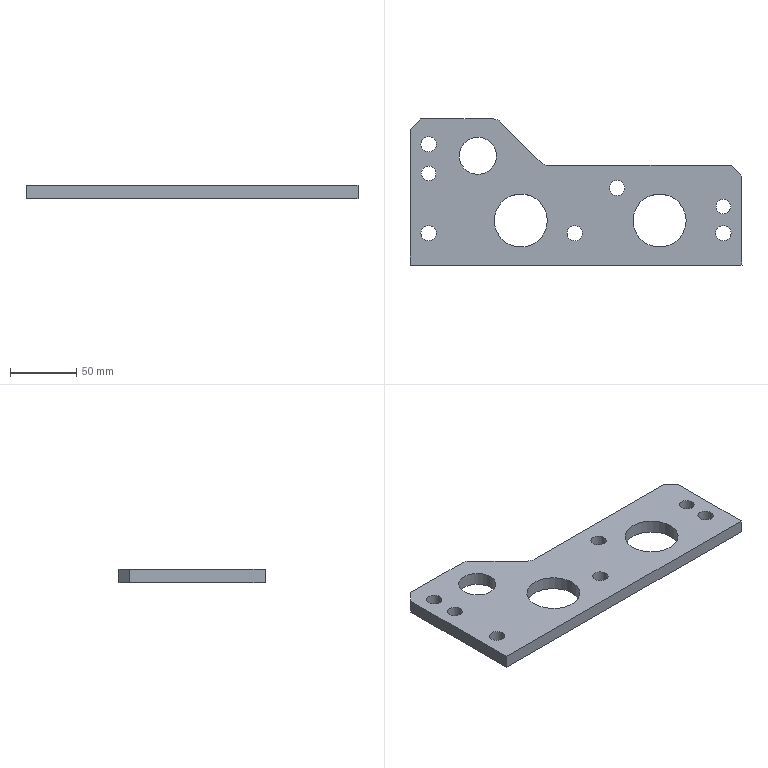Part | STEP file | lll_id4274_x_t | 1 solid | 22 faces | box 250 x 110 x 10 mm | volume 177692 mm3 | cylinder 12 | plane 10 | commonest cylinder face diameters 11.509 x5 11 x2 16 x2 40 x2 28 x1
STEP:
#1=CARTESIAN_POINT('',(3220.278,-130.093,-35.));
#2=VERTEX_POINT('',#1);
#3=CARTESIAN_POINT('',(3220.278,-130.093,-45.));
#4=VERTEX_POINT('',#3);
#5=CARTESIAN_POINT('',(3220.278,-130.093,-35.));
#6=DIRECTION('',(0.,0.,-1.));
#7=VECTOR('',#6,1.);
#8=LINE('',#5,#7);
#9=EDGE_CURVE('',#2,#4,#8,.T.);
#10=ORIENTED_EDGE('',*,*,#9,.F.);
#11=CARTESIAN_POINT('',(3250.592,-160.407,-35.));
#12=VERTEX_POINT('',#11);
#13=CARTESIAN_POINT('',(3285.935,-195.75,-35.));
#14=DIRECTION('',(0.7071,-0.7071,0.));
#15=VECTOR('',#14,1.);
#16=LINE('',#13,#15);
#17=EDGE_CURVE('',#2,#12,#16,.T.);
#18=ORIENTED_EDGE('',*,*,#17,.T.);
#19=CARTESIAN_POINT('',(3250.592,-160.407,-45.));
#20=VERTEX_POINT('',#19);
#21=CARTESIAN_POINT('',(3250.592,-160.407,-35.));
#22=DIRECTION('',(0.,0.,-1.));
#23=VECTOR('',#22,1.);
#24=LINE('',#21,#23);
#25=EDGE_CURVE('',#12,#20,#24,.T.);
#26=ORIENTED_EDGE('',*,*,#25,.T.);
#27=CARTESIAN_POINT('',(3434.56,-344.374,-45.));
#28=DIRECTION('',(0.7071,-0.7071,0.));
#29=VECTOR('',#28,1.);
#30=LINE('',#27,#29);
#31=EDGE_CURVE('',#4,#20,#30,.T.);
#32=ORIENTED_EDGE('',*,*,#31,.F.);
#33=EDGE_LOOP('',(#10,#18,#26,#32));
#34=FACE_OUTER_BOUND('',#33,.T.);
#35=CARTESIAN_POINT('',(3285.935,-195.75,-35.));
#36=DIRECTION('',(-0.7071,-0.7071,0.));
#37=DIRECTION('',(-0.7071,0.7071,0.));
#38=AXIS2_PLACEMENT_3D('',#35,#36,#37);
#39=PLANE('',#38);
#40=ADVANCED_FACE('',(#34),#39,.F.);
#41=ORIENTED_EDGE('',*,*,#25,.F.);
#42=CARTESIAN_POINT('',(3256.249,-162.75,-35.));
#43=VERTEX_POINT('',#42);
#44=CARTESIAN_POINT('',(3256.249,-154.75,-35.));
#45=DIRECTION('',(0.,0.,1.));
#46=DIRECTION('',(-1.,0.,0.));
#47=AXIS2_PLACEMENT_3D('',#44,#45,#46);
#48=CIRCLE('',#47,8.);
#49=EDGE_CURVE('',#12,#43,#48,.T.);
#50=ORIENTED_EDGE('',*,*,#49,.T.);
#51=CARTESIAN_POINT('',(3256.249,-162.75,-45.));
#52=VERTEX_POINT('',#51);
#53=CARTESIAN_POINT('',(3256.249,-162.75,-35.));
#54=DIRECTION('',(0.,0.,-1.));
#55=VECTOR('',#54,1.);
#56=LINE('',#53,#55);
#57=EDGE_CURVE('',#43,#52,#56,.T.);
#58=ORIENTED_EDGE('',*,*,#57,.T.);
#59=CARTESIAN_POINT('',(3256.249,-154.75,-45.));
#60=DIRECTION('',(0.,0.,1.));
#61=DIRECTION('',(-1.,0.,0.));
#62=AXIS2_PLACEMENT_3D('',#59,#60,#61);
#63=CIRCLE('',#62,8.);
#64=EDGE_CURVE('',#20,#52,#63,.T.);
#65=ORIENTED_EDGE('',*,*,#64,.F.);
#66=EDGE_LOOP('',(#41,#50,#58,#65));
#67=FACE_OUTER_BOUND('',#66,.T.);
#68=CARTESIAN_POINT('',(3256.249,-154.75,-35.));
#69=DIRECTION('',(0.,0.,-1.));
#70=DIRECTION('',(-1.,0.,0.));
#71=AXIS2_PLACEMENT_3D('',#68,#69,#70);
#72=CYLINDRICAL_SURFACE('',#71,8.);
#73=ADVANCED_FACE('',(#67),#72,.F.);
#74=ORIENTED_EDGE('',*,*,#57,.F.);
#75=CARTESIAN_POINT('',(3393.935,-162.75,-35.));
#76=VERTEX_POINT('',#75);
#77=CARTESIAN_POINT('',(3266.435,-162.75,-35.));
#78=DIRECTION('',(-1.,0.,0.));
#79=VECTOR('',#78,1.);
#80=LINE('',#77,#79);
#81=EDGE_CURVE('',#76,#43,#80,.T.);
#82=ORIENTED_EDGE('',*,*,#81,.F.);
#83=CARTESIAN_POINT('',(3393.935,-162.75,-45.));
#84=VERTEX_POINT('',#83);
#85=CARTESIAN_POINT('',(3393.935,-162.75,-35.));
#86=DIRECTION('',(0.,0.,-1.));
#87=VECTOR('',#86,1.);
#88=LINE('',#85,#87);
#89=EDGE_CURVE('',#76,#84,#88,.T.);
#90=ORIENTED_EDGE('',*,*,#89,.T.);
#91=CARTESIAN_POINT('',(3266.435,-162.75,-45.));
#92=DIRECTION('',(-1.,0.,0.));
#93=VECTOR('',#92,1.);
#94=LINE('',#91,#93);
#95=EDGE_CURVE('',#84,#52,#94,.T.);
#96=ORIENTED_EDGE('',*,*,#95,.T.);
#97=EDGE_LOOP('',(#74,#82,#90,#96));
#98=FACE_OUTER_BOUND('',#97,.T.);
#99=CARTESIAN_POINT('',(3266.435,-162.75,-35.));
#100=DIRECTION('',(0.,-1.,0.));
#101=DIRECTION('',(-1.,0.,0.));
#102=AXIS2_PLACEMENT_3D('',#99,#100,#101);
#103=PLANE('',#102);
#104=ADVANCED_FACE('',(#98),#103,.F.);
#105=ORIENTED_EDGE('',*,*,#89,.F.);
#106=CARTESIAN_POINT('',(3401.935,-170.75,-35.));
#107=VERTEX_POINT('',#106);
#108=CARTESIAN_POINT('',(3356.435,-125.25,-35.));
#109=DIRECTION('',(0.7071,-0.7071,0.));
#110=VECTOR('',#109,1.);
#111=LINE('',#108,#110);
#112=EDGE_CURVE('',#76,#107,#111,.T.);
#113=ORIENTED_EDGE('',*,*,#112,.T.);
#114=CARTESIAN_POINT('',(3401.935,-170.75,-45.));
#115=VERTEX_POINT('',#114);
#116=CARTESIAN_POINT('',(3401.935,-170.75,-35.));
#117=DIRECTION('',(0.,0.,-1.));
#118=VECTOR('',#117,1.);
#119=LINE('',#116,#118);
#120=EDGE_CURVE('',#107,#115,#119,.T.);
#121=ORIENTED_EDGE('',*,*,#120,.T.);
#122=CARTESIAN_POINT('',(3505.06,-273.874,-45.));
#123=DIRECTION('',(0.7071,-0.7071,0.));
#124=VECTOR('',#123,1.);
#125=LINE('',#122,#124);
#126=EDGE_CURVE('',#84,#115,#125,.T.);
#127=ORIENTED_EDGE('',*,*,#126,.F.);
#128=EDGE_LOOP('',(#105,#113,#121,#127));
#129=FACE_OUTER_BOUND('',#128,.T.);
#130=CARTESIAN_POINT('',(3356.435,-125.25,-35.));
#131=DIRECTION('',(0.7071,0.7071,0.));
#132=DIRECTION('',(0.7071,-0.7071,0.));
#133=AXIS2_PLACEMENT_3D('',#130,#131,#132);
#134=PLANE('',#133);
#135=ADVANCED_FACE('',(#129),#134,.T.);
#136=ORIENTED_EDGE('',*,*,#120,.F.);
#137=CARTESIAN_POINT('',(3401.935,-237.75,-35.));
#138=VERTEX_POINT('',#137);
#139=CARTESIAN_POINT('',(3401.935,-215.25,-35.));
#140=DIRECTION('',(0.,-1.,0.));
#141=VECTOR('',#140,1.);
#142=LINE('',#139,#141);
#143=EDGE_CURVE('',#107,#138,#142,.T.);
#144=ORIENTED_EDGE('',*,*,#143,.T.);
#145=CARTESIAN_POINT('',(3401.935,-237.75,-45.));
#146=VERTEX_POINT('',#145);
#147=CARTESIAN_POINT('',(3401.935,-237.75,-35.));
#148=DIRECTION('',(0.,0.,-1.));
#149=VECTOR('',#148,1.);
#150=LINE('',#147,#149);
#151=EDGE_CURVE('',#138,#146,#150,.T.);
#152=ORIENTED_EDGE('',*,*,#151,.T.);
#153=CARTESIAN_POINT('',(3401.935,-198.7,-45.));
#154=DIRECTION('',(0.,-1.,0.));
#155=VECTOR('',#154,1.);
#156=LINE('',#153,#155);
#157=EDGE_CURVE('',#115,#146,#156,.T.);
#158=ORIENTED_EDGE('',*,*,#157,.F.);
#159=EDGE_LOOP('',(#136,#144,#152,#158));
#160=FACE_OUTER_BOUND('',#159,.T.);
#161=CARTESIAN_POINT('',(3401.935,-215.25,-35.));
#162=DIRECTION('',(1.,0.,0.));
#163=DIRECTION('',(0.,-1.,0.));
#164=AXIS2_PLACEMENT_3D('',#161,#162,#163);
#165=PLANE('',#164);
#166=ADVANCED_FACE('',(#160),#165,.T.);
#167=ORIENTED_EDGE('',*,*,#151,.F.);
#168=CARTESIAN_POINT('',(3151.935,-237.75,-35.));
#169=VERTEX_POINT('',#168);
#170=CARTESIAN_POINT('',(3266.435,-237.75,-35.));
#171=DIRECTION('',(-1.,0.,0.));
#172=VECTOR('',#171,1.);
#173=LINE('',#170,#172);
#174=EDGE_CURVE('',#138,#169,#173,.T.);
#175=ORIENTED_EDGE('',*,*,#174,.T.);
#176=CARTESIAN_POINT('',(3151.935,-237.75,-45.));
#177=VERTEX_POINT('',#176);
#178=CARTESIAN_POINT('',(3151.935,-237.75,-35.));
#179=DIRECTION('',(0.,0.,-1.));
#180=VECTOR('',#179,1.);
#181=LINE('',#178,#180);
#182=EDGE_CURVE('',#169,#177,#181,.T.);
#183=ORIENTED_EDGE('',*,*,#182,.T.);
#184=CARTESIAN_POINT('',(3580.234,-237.75,-45.));
#185=DIRECTION('',(-1.,0.,0.));
#186=VECTOR('',#185,1.);
#187=LINE('',#184,#186);
#188=EDGE_CURVE('',#146,#177,#187,.T.);
#189=ORIENTED_EDGE('',*,*,#188,.F.);
#190=EDGE_LOOP('',(#167,#175,#183,#189));
#191=FACE_OUTER_BOUND('',#190,.T.);
#192=CARTESIAN_POINT('',(3266.435,-237.75,-35.));
#193=DIRECTION('',(0.,-1.,0.));
#194=DIRECTION('',(-1.,0.,0.));
#195=AXIS2_PLACEMENT_3D('',#192,#193,#194);
#196=PLANE('',#195);
#197=ADVANCED_FACE('',(#191),#196,.T.);
#198=ORIENTED_EDGE('',*,*,#182,.F.);
#199=CARTESIAN_POINT('',(3151.935,-135.75,-35.));
#200=VERTEX_POINT('',#199);
#201=CARTESIAN_POINT('',(3151.935,-215.25,-35.));
#202=DIRECTION('',(0.,1.,0.));
#203=VECTOR('',#202,1.);
#204=LINE('',#201,#203);
#205=EDGE_CURVE('',#169,#200,#204,.T.);
#206=ORIENTED_EDGE('',*,*,#205,.T.);
#207=CARTESIAN_POINT('',(3151.935,-135.75,-45.));
#208=VERTEX_POINT('',#207);
#209=CARTESIAN_POINT('',(3151.935,-135.75,-35.));
#210=DIRECTION('',(0.,0.,-1.));
#211=VECTOR('',#210,1.);
#212=LINE('',#209,#211);
#213=EDGE_CURVE('',#200,#208,#212,.T.);
#214=ORIENTED_EDGE('',*,*,#213,.T.);
#215=CARTESIAN_POINT('',(3151.935,-198.7,-45.));
#216=DIRECTION('',(0.,1.,0.));
#217=VECTOR('',#216,1.);
#218=LINE('',#215,#217);
#219=EDGE_CURVE('',#177,#208,#218,.T.);
#220=ORIENTED_EDGE('',*,*,#219,.F.);
#221=EDGE_LOOP('',(#198,#206,#214,#220));
#222=FACE_OUTER_BOUND('',#221,.T.);
#223=CARTESIAN_POINT('',(3151.935,-215.25,-35.));
#224=DIRECTION('',(-1.,0.,0.));
#225=DIRECTION('',(0.,1.,0.));
#226=AXIS2_PLACEMENT_3D('',#223,#224,#225);
#227=PLANE('',#226);
#228=ADVANCED_FACE('',(#222),#227,.T.);
#229=ORIENTED_EDGE('',*,*,#213,.F.);
#230=CARTESIAN_POINT('',(3159.935,-127.75,-35.));
#231=VERTEX_POINT('',#230);
#232=CARTESIAN_POINT('',(3169.435,-118.25,-35.));
#233=DIRECTION('',(0.7071,0.7071,0.));
#234=VECTOR('',#233,1.);
#235=LINE('',#232,#234);
#236=EDGE_CURVE('',#200,#231,#235,.T.);
#237=ORIENTED_EDGE('',*,*,#236,.T.);
#238=CARTESIAN_POINT('',(3159.935,-127.75,-45.));
#239=VERTEX_POINT('',#238);
#240=CARTESIAN_POINT('',(3159.935,-127.75,-35.));
#241=DIRECTION('',(0.,0.,-1.));
#242=VECTOR('',#241,1.);
#243=LINE('',#240,#242);
#244=EDGE_CURVE('',#231,#239,#243,.T.);
#245=ORIENTED_EDGE('',*,*,#244,.T.);
#246=CARTESIAN_POINT('',(3334.61,46.924,-45.));
#247=DIRECTION('',(0.7071,0.7071,0.));
#248=VECTOR('',#247,1.);
#249=LINE('',#246,#248);
#250=EDGE_CURVE('',#208,#239,#249,.T.);
#251=ORIENTED_EDGE('',*,*,#250,.F.);
#252=EDGE_LOOP('',(#229,#237,#245,#251));
#253=FACE_OUTER_BOUND('',#252,.T.);
#254=CARTESIAN_POINT('',(3169.435,-118.25,-35.));
#255=DIRECTION('',(-0.7071,0.7071,0.));
#256=DIRECTION('',(0.7071,0.7071,0.));
#257=AXIS2_PLACEMENT_3D('',#254,#255,#256);
#258=PLANE('',#257);
#259=ADVANCED_FACE('',(#253),#258,.T.);
#260=ORIENTED_EDGE('',*,*,#244,.F.);
#261=CARTESIAN_POINT('',(3214.622,-127.75,-35.));
#262=VERTEX_POINT('',#261);
#263=CARTESIAN_POINT('',(3266.435,-127.75,-35.));
#264=DIRECTION('',(1.,0.,0.));
#265=VECTOR('',#264,1.);
#266=LINE('',#263,#265);
#267=EDGE_CURVE('',#231,#262,#266,.T.);
#268=ORIENTED_EDGE('',*,*,#267,.T.);
#269=CARTESIAN_POINT('',(3214.622,-127.75,-45.));
#270=VERTEX_POINT('',#269);
#271=CARTESIAN_POINT('',(3214.622,-127.75,-35.));
#272=DIRECTION('',(0.,0.,-1.));
#273=VECTOR('',#272,1.);
#274=LINE('',#271,#273);
#275=EDGE_CURVE('',#262,#270,#274,.T.);
#276=ORIENTED_EDGE('',*,*,#275,.T.);
#277=CARTESIAN_POINT('',(3580.234,-127.75,-45.));
#278=DIRECTION('',(1.,0.,0.));
#279=VECTOR('',#278,1.);
#280=LINE('',#277,#279);
#281=EDGE_CURVE('',#239,#270,#280,.T.);
#282=ORIENTED_EDGE('',*,*,#281,.F.);
#283=EDGE_LOOP('',(#260,#268,#276,#282));
#284=FACE_OUTER_BOUND('',#283,.T.);
#285=CARTESIAN_POINT('',(3266.435,-127.75,-35.));
#286=DIRECTION('',(0.,-1.,0.));
#287=DIRECTION('',(-1.,0.,0.));
#288=AXIS2_PLACEMENT_3D('',#285,#286,#287);
#289=PLANE('',#288);
#290=ADVANCED_FACE('',(#284),#289,.F.);
#291=CARTESIAN_POINT('',(3382.181,-213.75,-45.));
#292=VERTEX_POINT('',#291);
#293=CARTESIAN_POINT('',(3387.935,-213.75,-45.));
#294=DIRECTION('',(0.,0.,-1.));
#295=DIRECTION('',(-1.,0.,0.));
#296=AXIS2_PLACEMENT_3D('',#293,#294,#295);
#297=CIRCLE('',#296,5.755);
#298=EDGE_CURVE('',#292,#292,#297,.T.);
#299=ORIENTED_EDGE('',*,*,#298,.T.);
#300=EDGE_LOOP('',(#299));
#301=FACE_BOUND('',#300,.T.);
#302=CARTESIAN_POINT('',(3382.181,-213.75,-35.));
#303=VERTEX_POINT('',#302);
#304=CARTESIAN_POINT('',(3387.935,-213.75,-35.));
#305=DIRECTION('',(0.,0.,-1.));
#306=DIRECTION('',(-1.,0.,0.));
#307=AXIS2_PLACEMENT_3D('',#304,#305,#306);
#308=CIRCLE('',#307,5.755);
#309=EDGE_CURVE('',#303,#303,#308,.T.);
#310=ORIENTED_EDGE('',*,*,#309,.F.);
#311=EDGE_LOOP('',(#310));
#312=FACE_BOUND('',#311,.T.);
#313=CARTESIAN_POINT('',(3387.935,-213.75,-35.));
#314=DIRECTION('',(0.,0.,-1.));
#315=DIRECTION('',(-1.,0.,0.));
#316=AXIS2_PLACEMENT_3D('',#313,#314,#315);
#317=CYLINDRICAL_SURFACE('',#316,5.755);
#318=ADVANCED_FACE('',(#301,#312),#317,.F.);
#319=CARTESIAN_POINT('',(3382.435,-193.75,-45.));
#320=VERTEX_POINT('',#319);
#321=CARTESIAN_POINT('',(3387.935,-193.75,-45.));
#322=DIRECTION('',(0.,0.,-1.));
#323=DIRECTION('',(-1.,0.,0.));
#324=AXIS2_PLACEMENT_3D('',#321,#322,#323);
#325=CIRCLE('',#324,5.5);
#326=EDGE_CURVE('',#320,#320,#325,.T.);
#327=ORIENTED_EDGE('',*,*,#326,.T.);
#328=EDGE_LOOP('',(#327));
#329=FACE_BOUND('',#328,.T.);
#330=CARTESIAN_POINT('',(3382.435,-193.75,-35.));
#331=VERTEX_POINT('',#330);
#332=CARTESIAN_POINT('',(3387.935,-193.75,-35.));
#333=DIRECTION('',(0.,0.,-1.));
#334=DIRECTION('',(-1.,0.,0.));
#335=AXIS2_PLACEMENT_3D('',#332,#333,#334);
#336=CIRCLE('',#335,5.5);
#337=EDGE_CURVE('',#331,#331,#336,.T.);
#338=ORIENTED_EDGE('',*,*,#337,.F.);
#339=EDGE_LOOP('',(#338));
#340=FACE_BOUND('',#339,.T.);
#341=CARTESIAN_POINT('',(3387.935,-193.75,-35.));
#342=DIRECTION('',(0.,0.,-1.));
#343=DIRECTION('',(-1.,0.,0.));
#344=AXIS2_PLACEMENT_3D('',#341,#342,#343);
#345=CYLINDRICAL_SURFACE('',#344,5.5);
#346=ADVANCED_FACE('',(#329,#340),#345,.F.);
#347=CARTESIAN_POINT('',(3302.181,-179.75,-45.));
#348=VERTEX_POINT('',#347);
#349=CARTESIAN_POINT('',(3307.935,-179.75,-45.));
#350=DIRECTION('',(0.,0.,-1.));
#351=DIRECTION('',(-1.,0.,0.));
#352=AXIS2_PLACEMENT_3D('',#349,#350,#351);
#353=CIRCLE('',#352,5.755);
#354=EDGE_CURVE('',#348,#348,#353,.T.);
#355=ORIENTED_EDGE('',*,*,#354,.T.);
#356=EDGE_LOOP('',(#355));
#357=FACE_BOUND('',#356,.T.);
#358=CARTESIAN_POINT('',(3302.181,-179.75,-35.));
#359=VERTEX_POINT('',#358);
#360=CARTESIAN_POINT('',(3307.935,-179.75,-35.));
#361=DIRECTION('',(0.,0.,-1.));
#362=DIRECTION('',(-1.,0.,0.));
#363=AXIS2_PLACEMENT_3D('',#360,#361,#362);
#364=CIRCLE('',#363,5.755);
#365=EDGE_CURVE('',#359,#359,#364,.T.);
#366=ORIENTED_EDGE('',*,*,#365,.F.);
#367=EDGE_LOOP('',(#366));
#368=FACE_BOUND('',#367,.T.);
#369=CARTESIAN_POINT('',(3307.935,-179.75,-35.));
#370=DIRECTION('',(0.,0.,-1.));
#371=DIRECTION('',(-1.,0.,0.));
#372=AXIS2_PLACEMENT_3D('',#369,#370,#371);
#373=CYLINDRICAL_SURFACE('',#372,5.755);
#374=ADVANCED_FACE('',(#357,#368),#373,.F.);
#375=CARTESIAN_POINT('',(3270.181,-213.75,-45.));
#376=VERTEX_POINT('',#375);
#377=CARTESIAN_POINT('',(3275.935,-213.75,-45.));
#378=DIRECTION('',(0.,0.,-1.));
#379=DIRECTION('',(-1.,0.,0.));
#380=AXIS2_PLACEMENT_3D('',#377,#378,#379);
#381=CIRCLE('',#380,5.755);
#382=EDGE_CURVE('',#376,#376,#381,.T.);
#383=ORIENTED_EDGE('',*,*,#382,.T.);
#384=EDGE_LOOP('',(#383));
#385=FACE_BOUND('',#384,.T.);
#386=CARTESIAN_POINT('',(3270.181,-213.75,-35.));
#387=VERTEX_POINT('',#386);
#388=CARTESIAN_POINT('',(3275.935,-213.75,-35.));
#389=DIRECTION('',(0.,0.,-1.));
#390=DIRECTION('',(-1.,0.,0.));
#391=AXIS2_PLACEMENT_3D('',#388,#389,#390);
#392=CIRCLE('',#391,5.755);
#393=EDGE_CURVE('',#387,#387,#392,.T.);
#394=ORIENTED_EDGE('',*,*,#393,.F.);
#395=EDGE_LOOP('',(#394));
#396=FACE_BOUND('',#395,.T.);
#397=CARTESIAN_POINT('',(3275.935,-213.75,-35.));
#398=DIRECTION('',(0.,0.,-1.));
#399=DIRECTION('',(-1.,0.,0.));
#400=AXIS2_PLACEMENT_3D('',#397,#398,#399);
#401=CYLINDRICAL_SURFACE('',#400,5.755);
#402=ADVANCED_FACE('',(#385,#396),#401,.F.);
#403=CARTESIAN_POINT('',(3160.435,-168.75,-45.));
#404=VERTEX_POINT('',#403);
#405=CARTESIAN_POINT('',(3165.935,-168.75,-45.));
#406=DIRECTION('',(0.,0.,-1.));
#407=DIRECTION('',(-1.,0.,0.));
#408=AXIS2_PLACEMENT_3D('',#405,#406,#407);
#409=CIRCLE('',#408,5.5);
#410=EDGE_CURVE('',#404,#404,#409,.T.);
#411=ORIENTED_EDGE('',*,*,#410,.T.);
#412=EDGE_LOOP('',(#411));
#413=FACE_BOUND('',#412,.T.);
#414=CARTESIAN_POINT('',(3160.435,-168.75,-35.));
#415=VERTEX_POINT('',#414);
#416=CARTESIAN_POINT('',(3165.935,-168.75,-35.));
#417=DIRECTION('',(0.,0.,-1.));
#418=DIRECTION('',(-1.,0.,0.));
#419=AXIS2_PLACEMENT_3D('',#416,#417,#418);
#420=CIRCLE('',#419,5.5);
#421=EDGE_CURVE('',#415,#415,#420,.T.);
#422=ORIENTED_EDGE('',*,*,#421,.F.);
#423=EDGE_LOOP('',(#422));
#424=FACE_BOUND('',#423,.T.);
#425=CARTESIAN_POINT('',(3165.935,-168.75,-35.));
#426=DIRECTION('',(0.,0.,-1.));
#427=DIRECTION('',(-1.,0.,0.));
#428=AXIS2_PLACEMENT_3D('',#425,#426,#427);
#429=CYLINDRICAL_SURFACE('',#428,5.5);
#430=ADVANCED_FACE('',(#413,#424),#429,.F.);
#431=CARTESIAN_POINT('',(3160.181,-213.75,-45.));
#432=VERTEX_POINT('',#431);
#433=CARTESIAN_POINT('',(3165.935,-213.75,-45.));
#434=DIRECTION('',(0.,0.,-1.));
#435=DIRECTION('',(-1.,0.,0.));
#436=AXIS2_PLACEMENT_3D('',#433,#434,#435);
#437=CIRCLE('',#436,5.755);
#438=EDGE_CURVE('',#432,#432,#437,.T.);
#439=ORIENTED_EDGE('',*,*,#438,.T.);
#440=EDGE_LOOP('',(#439));
#441=FACE_BOUND('',#440,.T.);
#442=CARTESIAN_POINT('',(3160.181,-213.75,-35.));
#443=VERTEX_POINT('',#442);
#444=CARTESIAN_POINT('',(3165.935,-213.75,-35.));
#445=DIRECTION('',(0.,0.,-1.));
#446=DIRECTION('',(-1.,0.,0.));
#447=AXIS2_PLACEMENT_3D('',#444,#445,#446);
#448=CIRCLE('',#447,5.755);
#449=EDGE_CURVE('',#443,#443,#448,.T.);
#450=ORIENTED_EDGE('',*,*,#449,.F.);
#451=EDGE_LOOP('',(#450));
#452=FACE_BOUND('',#451,.T.);
#453=CARTESIAN_POINT('',(3165.935,-213.75,-35.));
#454=DIRECTION('',(0.,0.,-1.));
#455=DIRECTION('',(-1.,0.,0.));
#456=AXIS2_PLACEMENT_3D('',#453,#454,#455);
#457=CYLINDRICAL_SURFACE('',#456,5.755);
#458=ADVANCED_FACE('',(#441,#452),#457,.F.);
#459=CARTESIAN_POINT('',(3160.181,-146.75,-45.));
#460=VERTEX_POINT('',#459);
#461=CARTESIAN_POINT('',(3165.935,-146.75,-45.));
#462=DIRECTION('',(0.,0.,-1.));
#463=DIRECTION('',(-1.,0.,0.));
#464=AXIS2_PLACEMENT_3D('',#461,#462,#463);
#465=CIRCLE('',#464,5.755);
#466=EDGE_CURVE('',#460,#460,#465,.T.);
#467=ORIENTED_EDGE('',*,*,#466,.T.);
#468=EDGE_LOOP('',(#467));
#469=FACE_BOUND('',#468,.T.);
#470=CARTESIAN_POINT('',(3160.181,-146.75,-35.));
#471=VERTEX_POINT('',#470);
#472=CARTESIAN_POINT('',(3165.935,-146.75,-35.));
#473=DIRECTION('',(0.,0.,-1.));
#474=DIRECTION('',(-1.,0.,0.));
#475=AXIS2_PLACEMENT_3D('',#472,#473,#474);
#476=CIRCLE('',#475,5.755);
#477=EDGE_CURVE('',#471,#471,#476,.T.);
#478=ORIENTED_EDGE('',*,*,#477,.F.);
#479=EDGE_LOOP('',(#478));
#480=FACE_BOUND('',#479,.T.);
#481=CARTESIAN_POINT('',(3165.935,-146.75,-35.));
#482=DIRECTION('',(0.,0.,-1.));
#483=DIRECTION('',(-1.,0.,0.));
#484=AXIS2_PLACEMENT_3D('',#481,#482,#483);
#485=CYLINDRICAL_SURFACE('',#484,5.755);
#486=ADVANCED_FACE('',(#469,#480),#485,.F.);
#487=CARTESIAN_POINT('',(3214.622,-135.75,-35.));
#488=DIRECTION('',(0.,0.,-1.));
#489=DIRECTION('',(-1.,0.,0.));
#490=AXIS2_PLACEMENT_3D('',#487,#488,#489);
#491=CIRCLE('',#490,8.);
#492=EDGE_CURVE('',#262,#2,#491,.T.);
#493=ORIENTED_EDGE('',*,*,#492,.T.);
#494=ORIENTED_EDGE('',*,*,#9,.T.);
#495=CARTESIAN_POINT('',(3214.622,-135.75,-45.));
#496=DIRECTION('',(0.,0.,-1.));
#497=DIRECTION('',(-1.,0.,0.));
#498=AXIS2_PLACEMENT_3D('',#495,#496,#497);
#499=CIRCLE('',#498,8.);
#500=EDGE_CURVE('',#270,#4,#499,.T.);
#501=ORIENTED_EDGE('',*,*,#500,.F.);
#502=ORIENTED_EDGE('',*,*,#275,.F.);
#503=EDGE_LOOP('',(#493,#494,#501,#502));
#504=FACE_OUTER_BOUND('',#503,.T.);
#505=CARTESIAN_POINT('',(3214.622,-135.75,-35.));
#506=DIRECTION('',(0.,0.,-1.));
#507=DIRECTION('',(-1.,0.,0.));
#508=AXIS2_PLACEMENT_3D('',#505,#506,#507);
#509=CYLINDRICAL_SURFACE('',#508,8.);
#510=ADVANCED_FACE('',(#504),#509,.T.);
#511=CARTESIAN_POINT('',(3215.367,-204.288,-45.));
#512=VERTEX_POINT('',#511);
#513=CARTESIAN_POINT('',(3235.367,-204.288,-45.));
#514=DIRECTION('',(0.,0.,1.));
#515=DIRECTION('',(-1.,0.,0.));
#516=AXIS2_PLACEMENT_3D('',#513,#514,#515);
#517=CIRCLE('',#516,20.);
#518=EDGE_CURVE('',#512,#512,#517,.T.);
#519=ORIENTED_EDGE('',*,*,#518,.F.);
#520=EDGE_LOOP('',(#519));
#521=FACE_BOUND('',#520,.T.);
#522=CARTESIAN_POINT('',(3215.367,-204.288,-35.));
#523=VERTEX_POINT('',#522);
#524=CARTESIAN_POINT('',(3235.367,-204.288,-35.));
#525=DIRECTION('',(0.,0.,1.));
#526=DIRECTION('',(-1.,0.,0.));
#527=AXIS2_PLACEMENT_3D('',#524,#525,#526);
#528=CIRCLE('',#527,20.);
#529=EDGE_CURVE('',#523,#523,#528,.T.);
#530=ORIENTED_EDGE('',*,*,#529,.T.);
#531=EDGE_LOOP('',(#530));
#532=FACE_BOUND('',#531,.T.);
#533=CARTESIAN_POINT('',(3235.367,-204.288,-35.));
#534=DIRECTION('',(0.,0.,-1.));
#535=DIRECTION('',(-1.,0.,0.));
#536=AXIS2_PLACEMENT_3D('',#533,#534,#535);
#537=CYLINDRICAL_SURFACE('',#536,20.);
#538=ADVANCED_FACE('',(#521,#532),#537,.F.);
#539=CARTESIAN_POINT('',(3319.867,-204.288,-45.));
#540=VERTEX_POINT('',#539);
#541=CARTESIAN_POINT('',(3339.867,-204.288,-45.));
#542=DIRECTION('',(0.,0.,1.));
#543=DIRECTION('',(-1.,0.,0.));
#544=AXIS2_PLACEMENT_3D('',#541,#542,#543);
#545=CIRCLE('',#544,20.);
#546=EDGE_CURVE('',#540,#540,#545,.T.);
#547=ORIENTED_EDGE('',*,*,#546,.F.);
#548=EDGE_LOOP('',(#547));
#549=FACE_BOUND('',#548,.T.);
#550=CARTESIAN_POINT('',(3319.867,-204.288,-35.));
#551=VERTEX_POINT('',#550);
#552=CARTESIAN_POINT('',(3339.867,-204.288,-35.));
#553=DIRECTION('',(0.,0.,1.));
#554=DIRECTION('',(-1.,0.,0.));
#555=AXIS2_PLACEMENT_3D('',#552,#553,#554);
#556=CIRCLE('',#555,20.);
#557=EDGE_CURVE('',#551,#551,#556,.T.);
#558=ORIENTED_EDGE('',*,*,#557,.T.);
#559=EDGE_LOOP('',(#558));
#560=FACE_BOUND('',#559,.T.);
#561=CARTESIAN_POINT('',(3339.867,-204.288,-35.));
#562=DIRECTION('',(0.,0.,-1.));
#563=DIRECTION('',(-1.,0.,0.));
#564=AXIS2_PLACEMENT_3D('',#561,#562,#563);
#565=CYLINDRICAL_SURFACE('',#564,20.);
#566=ADVANCED_FACE('',(#549,#560),#565,.F.);
#567=CARTESIAN_POINT('',(3189.,-155.5,-45.));
#568=VERTEX_POINT('',#567);
#569=CARTESIAN_POINT('',(3203.,-155.5,-45.));
#570=DIRECTION('',(0.,0.,-1.));
#571=DIRECTION('',(-1.,0.,0.));
#572=AXIS2_PLACEMENT_3D('',#569,#570,#571);
#573=CIRCLE('',#572,14.);
#574=EDGE_CURVE('',#568,#568,#573,.T.);
#575=ORIENTED_EDGE('',*,*,#574,.T.);
#576=EDGE_LOOP('',(#575));
#577=FACE_BOUND('',#576,.T.);
#578=CARTESIAN_POINT('',(3189.,-155.5,-35.));
#579=VERTEX_POINT('',#578);
#580=CARTESIAN_POINT('',(3203.,-155.5,-35.));
#581=DIRECTION('',(0.,0.,-1.));
#582=DIRECTION('',(-1.,0.,0.));
#583=AXIS2_PLACEMENT_3D('',#580,#581,#582);
#584=CIRCLE('',#583,14.);
#585=EDGE_CURVE('',#579,#579,#584,.T.);
#586=ORIENTED_EDGE('',*,*,#585,.F.);
#587=EDGE_LOOP('',(#586));
#588=FACE_BOUND('',#587,.T.);
#589=CARTESIAN_POINT('',(3203.,-155.5,-35.));
#590=DIRECTION('',(0.,0.,-1.));
#591=DIRECTION('',(-1.,0.,0.));
#592=AXIS2_PLACEMENT_3D('',#589,#590,#591);
#593=CYLINDRICAL_SURFACE('',#592,14.);
#594=ADVANCED_FACE('',(#577,#588),#593,.F.);
#595=ORIENTED_EDGE('',*,*,#298,.F.);
#596=EDGE_LOOP('',(#595));
#597=FACE_BOUND('',#596,.T.);
#598=ORIENTED_EDGE('',*,*,#326,.F.);
#599=EDGE_LOOP('',(#598));
#600=FACE_BOUND('',#599,.T.);
#601=ORIENTED_EDGE('',*,*,#354,.F.);
#602=EDGE_LOOP('',(#601));
#603=FACE_BOUND('',#602,.T.);
#604=ORIENTED_EDGE('',*,*,#382,.F.);
#605=EDGE_LOOP('',(#604));
#606=FACE_BOUND('',#605,.T.);
#607=ORIENTED_EDGE('',*,*,#410,.F.);
#608=EDGE_LOOP('',(#607));
#609=FACE_BOUND('',#608,.T.);
#610=ORIENTED_EDGE('',*,*,#438,.F.);
#611=EDGE_LOOP('',(#610));
#612=FACE_BOUND('',#611,.T.);
#613=ORIENTED_EDGE('',*,*,#466,.F.);
#614=EDGE_LOOP('',(#613));
#615=FACE_BOUND('',#614,.T.);
#616=ORIENTED_EDGE('',*,*,#281,.T.);
#617=ORIENTED_EDGE('',*,*,#500,.T.);
#618=ORIENTED_EDGE('',*,*,#31,.T.);
#619=ORIENTED_EDGE('',*,*,#64,.T.);
#620=ORIENTED_EDGE('',*,*,#95,.F.);
#621=ORIENTED_EDGE('',*,*,#126,.T.);
#622=ORIENTED_EDGE('',*,*,#157,.T.);
#623=ORIENTED_EDGE('',*,*,#188,.T.);
#624=ORIENTED_EDGE('',*,*,#219,.T.);
#625=ORIENTED_EDGE('',*,*,#250,.T.);
#626=EDGE_LOOP('',(#616,#617,#618,#619,#620,#621,#622,#623,#624,#625));
#627=FACE_BOUND('',#626,.T.);
#628=ORIENTED_EDGE('',*,*,#518,.T.);
#629=EDGE_LOOP('',(#628));
#630=FACE_BOUND('',#629,.T.);
#631=ORIENTED_EDGE('',*,*,#546,.T.);
#632=EDGE_LOOP('',(#631));
#633=FACE_BOUND('',#632,.T.);
#634=ORIENTED_EDGE('',*,*,#574,.F.);
#635=EDGE_LOOP('',(#634));
#636=FACE_BOUND('',#635,.T.);
#637=CARTESIAN_POINT('',(3580.234,-198.7,-45.));
#638=DIRECTION('',(0.,0.,-1.));
#639=DIRECTION('',(0.,-1.,0.));
#640=AXIS2_PLACEMENT_3D('',#637,#638,#639);
#641=PLANE('',#640);
#642=ADVANCED_FACE('',(#597,#600,#603,#606,#609,#612,#615,#627,#630,#633,#636),#641,.T.);
#643=ORIENTED_EDGE('',*,*,#309,.T.);
#644=EDGE_LOOP('',(#643));
#645=FACE_BOUND('',#644,.T.);
#646=ORIENTED_EDGE('',*,*,#337,.T.);
#647=EDGE_LOOP('',(#646));
#648=FACE_BOUND('',#647,.T.);
#649=ORIENTED_EDGE('',*,*,#365,.T.);
#650=EDGE_LOOP('',(#649));
#651=FACE_BOUND('',#650,.T.);
#652=ORIENTED_EDGE('',*,*,#393,.T.);
#653=EDGE_LOOP('',(#652));
#654=FACE_BOUND('',#653,.T.);
#655=ORIENTED_EDGE('',*,*,#421,.T.);
#656=EDGE_LOOP('',(#655));
#657=FACE_BOUND('',#656,.T.);
#658=ORIENTED_EDGE('',*,*,#449,.T.);
#659=EDGE_LOOP('',(#658));
#660=FACE_BOUND('',#659,.T.);
#661=ORIENTED_EDGE('',*,*,#477,.T.);
#662=EDGE_LOOP('',(#661));
#663=FACE_BOUND('',#662,.T.);
#664=ORIENTED_EDGE('',*,*,#267,.F.);
#665=ORIENTED_EDGE('',*,*,#236,.F.);
#666=ORIENTED_EDGE('',*,*,#205,.F.);
#667=ORIENTED_EDGE('',*,*,#174,.F.);
#668=ORIENTED_EDGE('',*,*,#143,.F.);
#669=ORIENTED_EDGE('',*,*,#112,.F.);
#670=ORIENTED_EDGE('',*,*,#81,.T.);
#671=ORIENTED_EDGE('',*,*,#49,.F.);
#672=ORIENTED_EDGE('',*,*,#17,.F.);
#673=ORIENTED_EDGE('',*,*,#492,.F.);
#674=EDGE_LOOP('',(#664,#665,#666,#667,#668,#669,#670,#671,#672,#673));
#675=FACE_BOUND('',#674,.T.);
#676=ORIENTED_EDGE('',*,*,#529,.F.);
#677=EDGE_LOOP('',(#676));
#678=FACE_BOUND('',#677,.T.);
#679=ORIENTED_EDGE('',*,*,#557,.F.);
#680=EDGE_LOOP('',(#679));
#681=FACE_BOUND('',#680,.T.);
#682=ORIENTED_EDGE('',*,*,#585,.T.);
#683=EDGE_LOOP('',(#682));
#684=FACE_BOUND('',#683,.T.);
#685=CARTESIAN_POINT('',(3266.435,-215.25,-35.));
#686=DIRECTION('',(0.,0.,-1.));
#687=DIRECTION('',(1.,0.,0.));
#688=AXIS2_PLACEMENT_3D('',#685,#686,#687);
#689=PLANE('',#688);
#690=ADVANCED_FACE('',(#645,#648,#651,#654,#657,#660,#663,#675,#678,#681,#684),#689,.F.);
#691=CLOSED_SHELL('',(#40,#73,#104,#135,#166,#197,#228,#259,#290,#318,#346,#374,#402,#430,#458,#486,#510,#538,#566,#594,#642,#690));
#692=MANIFOLD_SOLID_BREP('',#691);
#693=(LENGTH_UNIT()NAMED_UNIT(*)SI_UNIT(.MILLI.,.METRE.));
#694=UNCERTAINTY_MEASURE_WITH_UNIT(LENGTH_MEASURE(0.00002),#693,'','');
#695=(NAMED_UNIT(*)PLANE_ANGLE_UNIT()SI_UNIT($,.RADIAN.));
#696=PLANE_ANGLE_MEASURE_WITH_UNIT(PLANE_ANGLE_MEASURE(0.01745),#695);
#697=DIMENSIONAL_EXPONENTS(0.,0.,0.,0.,0.,0.,0.);
#698=(CONVERSION_BASED_UNIT('DEGREE',#696)NAMED_UNIT(#697)PLANE_ANGLE_UNIT());
#699=(NAMED_UNIT(*)SI_UNIT($,.STERADIAN.)SOLID_ANGLE_UNIT());
#700=(GEOMETRIC_REPRESENTATION_CONTEXT(3)GLOBAL_UNCERTAINTY_ASSIGNED_CONTEXT((#694))GLOBAL_UNIT_ASSIGNED_CONTEXT((#693,#698,#699))REPRESENTATION_CONTEXT('',''));
#701=ADVANCED_BREP_SHAPE_REPRESENTATION('',(#692),#700);